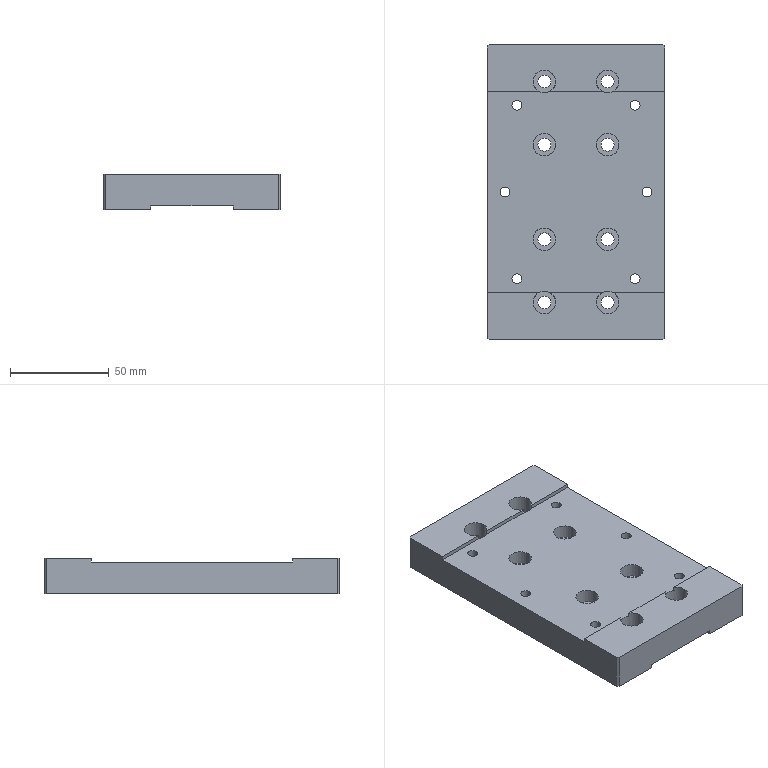Part | NX | features BREP 1 | 1 solid | 74 faces | box 90 x 150 x 18 mm | volume 201579 mm3 | cylinder 44 | plane 30 | commonest cylinder face diameters 6.6 x16 11.5 x16 5 x12